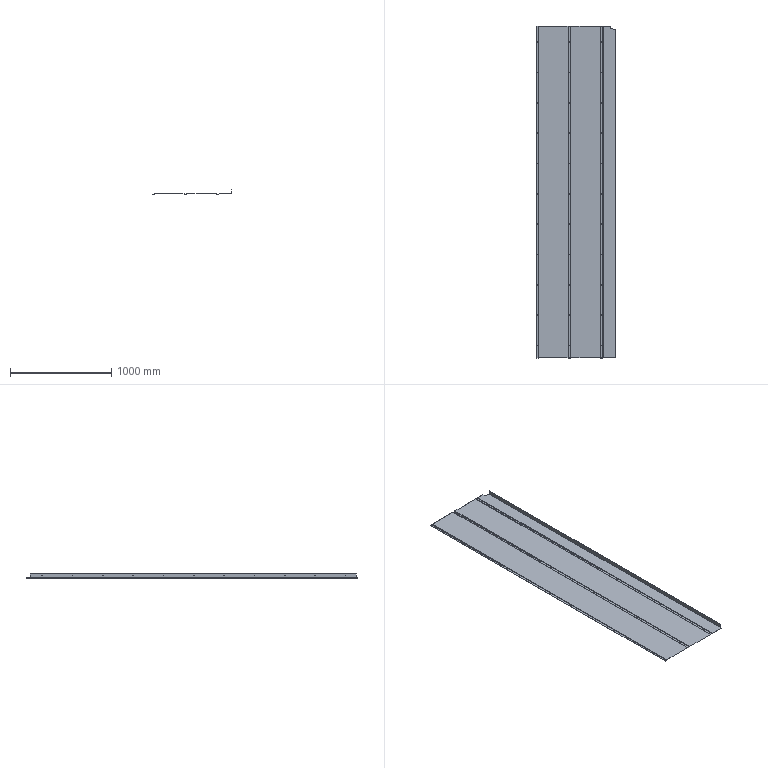Part | STEP file | TS-S98 | 1 solid | 191 faces | box 790 x 3283 x 43 mm | volume 3281115 mm3 | cylinder 113 | plane 78 | commonest cylinder face diameters 5.4 x88 0.4 x11 2.8 x11 10 x1 14 x1 16 x1